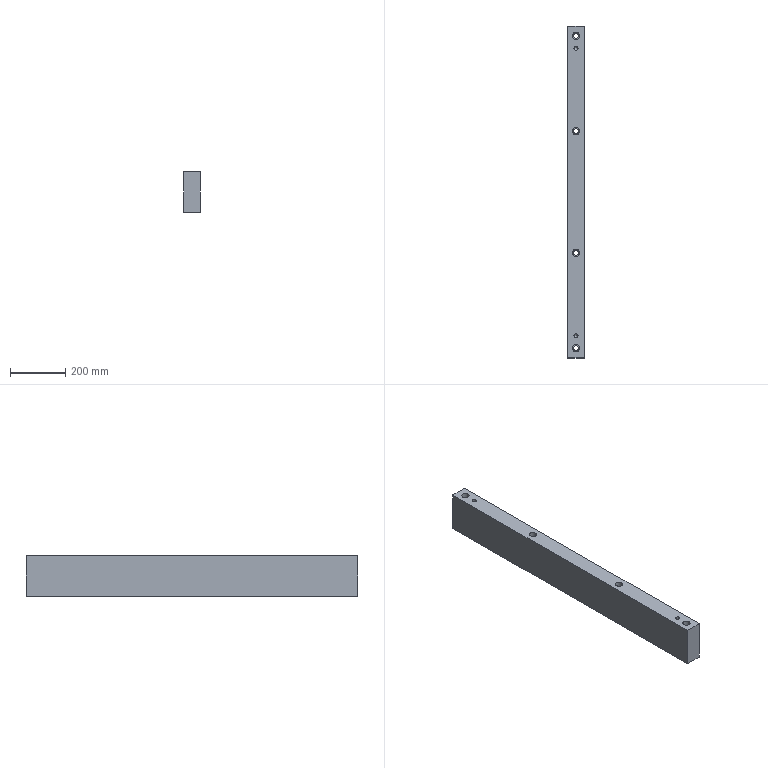Part | STEP file | lll_id1774_x_t | 1 solid | 22 faces | box 60 x 1200 x 147.5 mm | volume 10381772 mm3 | plane 10 | cylinder 10 | cone 2 | commonest cylinder face diameters 18.009 x4 26.008 x4 14.506 x2
STEP:
#1=CARTESIAN_POINT('',(1069.688,-520.,370.));
#2=VERTEX_POINT('',#1);
#3=CARTESIAN_POINT('',(1062.435,-520.,370.));
#4=DIRECTION('',(0.,0.,-1.));
#5=DIRECTION('',(1.,0.,0.));
#6=AXIS2_PLACEMENT_3D('',#3,#4,#5);
#7=CIRCLE('',#6,7.253);
#8=EDGE_CURVE('',#2,#2,#7,.T.);
#9=ORIENTED_EDGE('',*,*,#8,.T.);
#10=EDGE_LOOP('',(#9));
#11=FACE_BOUND('',#10,.T.);
#12=CARTESIAN_POINT('',(1069.688,520.,370.));
#13=VERTEX_POINT('',#12);
#14=CARTESIAN_POINT('',(1062.435,520.,370.));
#15=DIRECTION('',(0.,0.,1.));
#16=DIRECTION('',(1.,0.,0.));
#17=AXIS2_PLACEMENT_3D('',#14,#15,#16);
#18=CIRCLE('',#17,7.253);
#19=EDGE_CURVE('',#13,#13,#18,.T.);
#20=ORIENTED_EDGE('',*,*,#19,.F.);
#21=EDGE_LOOP('',(#20));
#22=FACE_BOUND('',#21,.T.);
#23=CARTESIAN_POINT('',(1075.439,565.,370.));
#24=VERTEX_POINT('',#23);
#25=CARTESIAN_POINT('',(1062.435,565.,370.));
#26=DIRECTION('',(0.,0.,1.));
#27=DIRECTION('',(1.,0.,0.));
#28=AXIS2_PLACEMENT_3D('',#25,#26,#27);
#29=CIRCLE('',#28,13.004);
#30=EDGE_CURVE('',#24,#24,#29,.T.);
#31=ORIENTED_EDGE('',*,*,#30,.F.);
#32=EDGE_LOOP('',(#31));
#33=FACE_BOUND('',#32,.T.);
#34=CARTESIAN_POINT('',(1032.435,600.,370.));
#35=VERTEX_POINT('',#34);
#36=CARTESIAN_POINT('',(1092.435,600.,370.));
#37=VERTEX_POINT('',#36);
#38=CARTESIAN_POINT('',(3278.751,600.,370.));
#39=DIRECTION('',(1.,0.,0.));
#40=VECTOR('',#39,1.);
#41=LINE('',#38,#40);
#42=EDGE_CURVE('',#35,#37,#41,.T.);
#43=ORIENTED_EDGE('',*,*,#42,.F.);
#44=CARTESIAN_POINT('',(1032.435,-600.,370.));
#45=VERTEX_POINT('',#44);
#46=CARTESIAN_POINT('',(1032.435,0.,370.));
#47=DIRECTION('',(0.,1.,0.));
#48=VECTOR('',#47,1.);
#49=LINE('',#46,#48);
#50=EDGE_CURVE('',#45,#35,#49,.T.);
#51=ORIENTED_EDGE('',*,*,#50,.F.);
#52=CARTESIAN_POINT('',(1092.435,-600.,370.));
#53=VERTEX_POINT('',#52);
#54=CARTESIAN_POINT('',(3278.751,-600.,370.));
#55=DIRECTION('',(-1.,0.,0.));
#56=VECTOR('',#55,1.);
#57=LINE('',#54,#56);
#58=EDGE_CURVE('',#53,#45,#57,.T.);
#59=ORIENTED_EDGE('',*,*,#58,.F.);
#60=CARTESIAN_POINT('',(1092.435,1.,370.));
#61=DIRECTION('',(0.,-1.,0.));
#62=VECTOR('',#61,1.);
#63=LINE('',#60,#62);
#64=EDGE_CURVE('',#37,#53,#63,.T.);
#65=ORIENTED_EDGE('',*,*,#64,.F.);
#66=EDGE_LOOP('',(#43,#51,#59,#65));
#67=FACE_BOUND('',#66,.T.);
#68=CARTESIAN_POINT('',(1075.439,-565.,370.));
#69=VERTEX_POINT('',#68);
#70=CARTESIAN_POINT('',(1062.435,-565.,370.));
#71=DIRECTION('',(0.,0.,-1.));
#72=DIRECTION('',(1.,0.,0.));
#73=AXIS2_PLACEMENT_3D('',#70,#71,#72);
#74=CIRCLE('',#73,13.004);
#75=EDGE_CURVE('',#69,#69,#74,.T.);
#76=ORIENTED_EDGE('',*,*,#75,.T.);
#77=EDGE_LOOP('',(#76));
#78=FACE_BOUND('',#77,.T.);
#79=CARTESIAN_POINT('',(1075.439,-220.,370.));
#80=VERTEX_POINT('',#79);
#81=CARTESIAN_POINT('',(1062.435,-220.,370.));
#82=DIRECTION('',(0.,0.,-1.));
#83=DIRECTION('',(1.,0.,0.));
#84=AXIS2_PLACEMENT_3D('',#81,#82,#83);
#85=CIRCLE('',#84,13.004);
#86=EDGE_CURVE('',#80,#80,#85,.T.);
#87=ORIENTED_EDGE('',*,*,#86,.T.);
#88=EDGE_LOOP('',(#87));
#89=FACE_BOUND('',#88,.T.);
#90=CARTESIAN_POINT('',(1075.439,220.,370.));
#91=VERTEX_POINT('',#90);
#92=CARTESIAN_POINT('',(1062.435,220.,370.));
#93=DIRECTION('',(0.,0.,1.));
#94=DIRECTION('',(1.,0.,0.));
#95=AXIS2_PLACEMENT_3D('',#92,#93,#94);
#96=CIRCLE('',#95,13.004);
#97=EDGE_CURVE('',#91,#91,#96,.T.);
#98=ORIENTED_EDGE('',*,*,#97,.F.);
#99=EDGE_LOOP('',(#98));
#100=FACE_BOUND('',#99,.T.);
#101=CARTESIAN_POINT('',(3278.751,1.,370.));
#102=DIRECTION('',(0.,0.,-1.));
#103=DIRECTION('',(-1.,0.,0.));
#104=AXIS2_PLACEMENT_3D('',#101,#102,#103);
#105=PLANE('',#104);
#106=ADVANCED_FACE('',(#11,#22,#33,#67,#78,#89,#100),#105,.F.);
#107=CARTESIAN_POINT('',(1071.44,-220.,222.5));
#108=VERTEX_POINT('',#107);
#109=CARTESIAN_POINT('',(1062.435,-220.,222.5));
#110=DIRECTION('',(0.,0.,1.));
#111=DIRECTION('',(1.,0.,0.));
#112=AXIS2_PLACEMENT_3D('',#109,#110,#111);
#113=CIRCLE('',#112,9.005);
#114=EDGE_CURVE('',#108,#108,#113,.T.);
#115=ORIENTED_EDGE('',*,*,#114,.T.);
#116=EDGE_LOOP('',(#115));
#117=FACE_BOUND('',#116,.T.);
#118=CARTESIAN_POINT('',(1032.435,600.,222.5));
#119=VERTEX_POINT('',#118);
#120=CARTESIAN_POINT('',(1092.435,600.,222.5));
#121=VERTEX_POINT('',#120);
#122=CARTESIAN_POINT('',(-2877.565,600.,222.5));
#123=DIRECTION('',(1.,0.,0.));
#124=VECTOR('',#123,1.);
#125=LINE('',#122,#124);
#126=EDGE_CURVE('',#119,#121,#125,.T.);
#127=ORIENTED_EDGE('',*,*,#126,.T.);
#128=CARTESIAN_POINT('',(1092.435,-600.,222.5));
#129=VERTEX_POINT('',#128);
#130=CARTESIAN_POINT('',(1092.435,600.,222.5));
#131=DIRECTION('',(0.,-1.,0.));
#132=VECTOR('',#131,1.);
#133=LINE('',#130,#132);
#134=EDGE_CURVE('',#121,#129,#133,.T.);
#135=ORIENTED_EDGE('',*,*,#134,.T.);
#136=CARTESIAN_POINT('',(1032.435,-600.,222.5));
#137=VERTEX_POINT('',#136);
#138=CARTESIAN_POINT('',(1092.435,-600.,222.5));
#139=DIRECTION('',(-1.,0.,0.));
#140=VECTOR('',#139,1.);
#141=LINE('',#138,#140);
#142=EDGE_CURVE('',#129,#137,#141,.T.);
#143=ORIENTED_EDGE('',*,*,#142,.T.);
#144=CARTESIAN_POINT('',(1032.435,1.,222.5));
#145=DIRECTION('',(0.,-1.,0.));
#146=VECTOR('',#145,1.);
#147=LINE('',#144,#146);
#148=EDGE_CURVE('',#119,#137,#147,.T.);
#149=ORIENTED_EDGE('',*,*,#148,.F.);
#150=EDGE_LOOP('',(#127,#135,#143,#149));
#151=FACE_BOUND('',#150,.T.);
#152=CARTESIAN_POINT('',(1071.44,-565.,222.5));
#153=VERTEX_POINT('',#152);
#154=CARTESIAN_POINT('',(1062.435,-565.,222.5));
#155=DIRECTION('',(0.,0.,1.));
#156=DIRECTION('',(1.,0.,0.));
#157=AXIS2_PLACEMENT_3D('',#154,#155,#156);
#158=CIRCLE('',#157,9.005);
#159=EDGE_CURVE('',#153,#153,#158,.T.);
#160=ORIENTED_EDGE('',*,*,#159,.T.);
#161=EDGE_LOOP('',(#160));
#162=FACE_BOUND('',#161,.T.);
#163=CARTESIAN_POINT('',(1071.44,220.,222.5));
#164=VERTEX_POINT('',#163);
#165=CARTESIAN_POINT('',(1062.435,220.,222.5));
#166=DIRECTION('',(0.,0.,-1.));
#167=DIRECTION('',(1.,0.,0.));
#168=AXIS2_PLACEMENT_3D('',#165,#166,#167);
#169=CIRCLE('',#168,9.005);
#170=EDGE_CURVE('',#164,#164,#169,.T.);
#171=ORIENTED_EDGE('',*,*,#170,.F.);
#172=EDGE_LOOP('',(#171));
#173=FACE_BOUND('',#172,.T.);
#174=CARTESIAN_POINT('',(1071.44,565.,222.5));
#175=VERTEX_POINT('',#174);
#176=CARTESIAN_POINT('',(1062.435,565.,222.5));
#177=DIRECTION('',(0.,0.,-1.));
#178=DIRECTION('',(1.,0.,0.));
#179=AXIS2_PLACEMENT_3D('',#176,#177,#178);
#180=CIRCLE('',#179,9.005);
#181=EDGE_CURVE('',#175,#175,#180,.T.);
#182=ORIENTED_EDGE('',*,*,#181,.F.);
#183=EDGE_LOOP('',(#182));
#184=FACE_BOUND('',#183,.T.);
#185=CARTESIAN_POINT('',(3278.751,1.,222.5));
#186=DIRECTION('',(0.,0.,-1.));
#187=DIRECTION('',(-1.,0.,0.));
#188=AXIS2_PLACEMENT_3D('',#185,#186,#187);
#189=PLANE('',#188);
#190=ADVANCED_FACE('',(#117,#151,#162,#173,#184),#189,.T.);
#191=ORIENTED_EDGE('',*,*,#134,.F.);
#192=CARTESIAN_POINT('',(1092.435,600.,360.));
#193=DIRECTION('',(0.,0.,-1.));
#194=VECTOR('',#193,1.);
#195=LINE('',#192,#194);
#196=EDGE_CURVE('',#37,#121,#195,.T.);
#197=ORIENTED_EDGE('',*,*,#196,.F.);
#198=ORIENTED_EDGE('',*,*,#64,.T.);
#199=CARTESIAN_POINT('',(1092.435,-600.,360.));
#200=DIRECTION('',(0.,0.,-1.));
#201=VECTOR('',#200,1.);
#202=LINE('',#199,#201);
#203=EDGE_CURVE('',#53,#129,#202,.T.);
#204=ORIENTED_EDGE('',*,*,#203,.T.);
#205=EDGE_LOOP('',(#191,#197,#198,#204));
#206=FACE_OUTER_BOUND('',#205,.T.);
#207=CARTESIAN_POINT('',(1092.435,600.,360.));
#208=DIRECTION('',(1.,0.,0.));
#209=DIRECTION('',(0.,0.,-1.));
#210=AXIS2_PLACEMENT_3D('',#207,#208,#209);
#211=PLANE('',#210);
#212=ADVANCED_FACE('',(#206),#211,.T.);
#213=CARTESIAN_POINT('',(1032.435,-600.,360.));
#214=DIRECTION('',(0.,0.,-1.));
#215=VECTOR('',#214,1.);
#216=LINE('',#213,#215);
#217=EDGE_CURVE('',#45,#137,#216,.T.);
#218=ORIENTED_EDGE('',*,*,#217,.T.);
#219=ORIENTED_EDGE('',*,*,#142,.F.);
#220=ORIENTED_EDGE('',*,*,#203,.F.);
#221=ORIENTED_EDGE('',*,*,#58,.T.);
#222=EDGE_LOOP('',(#218,#219,#220,#221));
#223=FACE_OUTER_BOUND('',#222,.T.);
#224=CARTESIAN_POINT('',(1092.435,-600.,360.));
#225=DIRECTION('',(0.,-1.,0.));
#226=DIRECTION('',(0.,0.,-1.));
#227=AXIS2_PLACEMENT_3D('',#224,#225,#226);
#228=PLANE('',#227);
#229=ADVANCED_FACE('',(#223),#228,.T.);
#230=CARTESIAN_POINT('',(1032.435,600.,360.));
#231=DIRECTION('',(0.,0.,1.));
#232=VECTOR('',#231,1.);
#233=LINE('',#230,#232);
#234=EDGE_CURVE('',#119,#35,#233,.T.);
#235=ORIENTED_EDGE('',*,*,#234,.T.);
#236=ORIENTED_EDGE('',*,*,#42,.T.);
#237=ORIENTED_EDGE('',*,*,#196,.T.);
#238=ORIENTED_EDGE('',*,*,#126,.F.);
#239=EDGE_LOOP('',(#235,#236,#237,#238));
#240=FACE_OUTER_BOUND('',#239,.T.);
#241=CARTESIAN_POINT('',(-2877.565,600.,360.));
#242=DIRECTION('',(0.,1.,0.));
#243=DIRECTION('',(0.,0.,1.));
#244=AXIS2_PLACEMENT_3D('',#241,#242,#243);
#245=PLANE('',#244);
#246=ADVANCED_FACE('',(#240),#245,.T.);
#247=ORIENTED_EDGE('',*,*,#148,.T.);
#248=ORIENTED_EDGE('',*,*,#217,.F.);
#249=ORIENTED_EDGE('',*,*,#50,.T.);
#250=ORIENTED_EDGE('',*,*,#234,.F.);
#251=EDGE_LOOP('',(#247,#248,#249,#250));
#252=FACE_OUTER_BOUND('',#251,.T.);
#253=CARTESIAN_POINT('',(1032.435,0.,291.25));
#254=DIRECTION('',(1.,0.,0.));
#255=DIRECTION('',(0.,0.,-1.));
#256=AXIS2_PLACEMENT_3D('',#253,#254,#255);
#257=PLANE('',#256);
#258=ADVANCED_FACE('',(#252),#257,.F.);
#259=CARTESIAN_POINT('',(1071.44,-565.,302.5));
#260=VERTEX_POINT('',#259);
#261=CARTESIAN_POINT('',(1062.435,-565.,302.5));
#262=DIRECTION('',(0.,0.,-1.));
#263=DIRECTION('',(1.,0.,0.));
#264=AXIS2_PLACEMENT_3D('',#261,#262,#263);
#265=CIRCLE('',#264,9.005);
#266=EDGE_CURVE('',#260,#260,#265,.T.);
#267=ORIENTED_EDGE('',*,*,#266,.F.);
#268=EDGE_LOOP('',(#267));
#269=FACE_BOUND('',#268,.T.);
#270=ORIENTED_EDGE('',*,*,#159,.F.);
#271=EDGE_LOOP('',(#270));
#272=FACE_BOUND('',#271,.T.);
#273=CARTESIAN_POINT('',(1062.435,-565.,420.));
#274=DIRECTION('',(0.,0.,-1.));
#275=DIRECTION('',(1.,0.,0.));
#276=AXIS2_PLACEMENT_3D('',#273,#274,#275);
#277=CYLINDRICAL_SURFACE('',#276,9.005);
#278=ADVANCED_FACE('',(#269,#272),#277,.F.);
#279=ORIENTED_EDGE('',*,*,#266,.T.);
#280=EDGE_LOOP('',(#279));
#281=FACE_BOUND('',#280,.T.);
#282=CARTESIAN_POINT('',(1075.439,-565.,302.5));
#283=VERTEX_POINT('',#282);
#284=CARTESIAN_POINT('',(1062.435,-565.,302.5));
#285=DIRECTION('',(0.,0.,-1.));
#286=DIRECTION('',(1.,0.,0.));
#287=AXIS2_PLACEMENT_3D('',#284,#285,#286);
#288=CIRCLE('',#287,13.004);
#289=EDGE_CURVE('',#283,#283,#288,.T.);
#290=ORIENTED_EDGE('',*,*,#289,.F.);
#291=EDGE_LOOP('',(#290));
#292=FACE_BOUND('',#291,.T.);
#293=CARTESIAN_POINT('',(2132.435,0.,302.5));
#294=DIRECTION('',(0.,0.,1.));
#295=DIRECTION('',(1.,0.,0.));
#296=AXIS2_PLACEMENT_3D('',#293,#294,#295);
#297=PLANE('',#296);
#298=ADVANCED_FACE('',(#281,#292),#297,.T.);
#299=ORIENTED_EDGE('',*,*,#289,.T.);
#300=EDGE_LOOP('',(#299));
#301=FACE_BOUND('',#300,.T.);
#302=ORIENTED_EDGE('',*,*,#75,.F.);
#303=EDGE_LOOP('',(#302));
#304=FACE_BOUND('',#303,.T.);
#305=CARTESIAN_POINT('',(1062.435,-565.,420.));
#306=DIRECTION('',(0.,0.,-1.));
#307=DIRECTION('',(1.,0.,0.));
#308=AXIS2_PLACEMENT_3D('',#305,#306,#307);
#309=CYLINDRICAL_SURFACE('',#308,13.004);
#310=ADVANCED_FACE('',(#301,#304),#309,.F.);
#311=CARTESIAN_POINT('',(1071.44,-220.,302.5));
#312=VERTEX_POINT('',#311);
#313=CARTESIAN_POINT('',(1062.435,-220.,302.5));
#314=DIRECTION('',(0.,0.,-1.));
#315=DIRECTION('',(1.,0.,0.));
#316=AXIS2_PLACEMENT_3D('',#313,#314,#315);
#317=CIRCLE('',#316,9.005);
#318=EDGE_CURVE('',#312,#312,#317,.T.);
#319=ORIENTED_EDGE('',*,*,#318,.F.);
#320=EDGE_LOOP('',(#319));
#321=FACE_BOUND('',#320,.T.);
#322=ORIENTED_EDGE('',*,*,#114,.F.);
#323=EDGE_LOOP('',(#322));
#324=FACE_BOUND('',#323,.T.);
#325=CARTESIAN_POINT('',(1062.435,-220.,420.));
#326=DIRECTION('',(0.,0.,-1.));
#327=DIRECTION('',(1.,0.,0.));
#328=AXIS2_PLACEMENT_3D('',#325,#326,#327);
#329=CYLINDRICAL_SURFACE('',#328,9.005);
#330=ADVANCED_FACE('',(#321,#324),#329,.F.);
#331=ORIENTED_EDGE('',*,*,#318,.T.);
#332=EDGE_LOOP('',(#331));
#333=FACE_BOUND('',#332,.T.);
#334=CARTESIAN_POINT('',(1075.439,-220.,302.5));
#335=VERTEX_POINT('',#334);
#336=CARTESIAN_POINT('',(1062.435,-220.,302.5));
#337=DIRECTION('',(0.,0.,-1.));
#338=DIRECTION('',(1.,0.,0.));
#339=AXIS2_PLACEMENT_3D('',#336,#337,#338);
#340=CIRCLE('',#339,13.004);
#341=EDGE_CURVE('',#335,#335,#340,.T.);
#342=ORIENTED_EDGE('',*,*,#341,.F.);
#343=EDGE_LOOP('',(#342));
#344=FACE_BOUND('',#343,.T.);
#345=CARTESIAN_POINT('',(2132.435,0.,302.5));
#346=DIRECTION('',(0.,0.,1.));
#347=DIRECTION('',(1.,0.,0.));
#348=AXIS2_PLACEMENT_3D('',#345,#346,#347);
#349=PLANE('',#348);
#350=ADVANCED_FACE('',(#333,#344),#349,.T.);
#351=ORIENTED_EDGE('',*,*,#341,.T.);
#352=EDGE_LOOP('',(#351));
#353=FACE_BOUND('',#352,.T.);
#354=ORIENTED_EDGE('',*,*,#86,.F.);
#355=EDGE_LOOP('',(#354));
#356=FACE_BOUND('',#355,.T.);
#357=CARTESIAN_POINT('',(1062.435,-220.,420.));
#358=DIRECTION('',(0.,0.,-1.));
#359=DIRECTION('',(1.,0.,0.));
#360=AXIS2_PLACEMENT_3D('',#357,#358,#359);
#361=CYLINDRICAL_SURFACE('',#360,13.004);
#362=ADVANCED_FACE('',(#353,#356),#361,.F.);
#363=CARTESIAN_POINT('',(1071.44,220.,302.5));
#364=VERTEX_POINT('',#363);
#365=CARTESIAN_POINT('',(1062.435,220.,302.5));
#366=DIRECTION('',(0.,0.,1.));
#367=DIRECTION('',(1.,0.,0.));
#368=AXIS2_PLACEMENT_3D('',#365,#366,#367);
#369=CIRCLE('',#368,9.005);
#370=EDGE_CURVE('',#364,#364,#369,.T.);
#371=ORIENTED_EDGE('',*,*,#370,.T.);
#372=EDGE_LOOP('',(#371));
#373=FACE_BOUND('',#372,.T.);
#374=ORIENTED_EDGE('',*,*,#170,.T.);
#375=EDGE_LOOP('',(#374));
#376=FACE_BOUND('',#375,.T.);
#377=CARTESIAN_POINT('',(1062.435,220.,420.));
#378=DIRECTION('',(0.,0.,-1.));
#379=DIRECTION('',(1.,0.,0.));
#380=AXIS2_PLACEMENT_3D('',#377,#378,#379);
#381=CYLINDRICAL_SURFACE('',#380,9.005);
#382=ADVANCED_FACE('',(#373,#376),#381,.F.);
#383=ORIENTED_EDGE('',*,*,#370,.F.);
#384=EDGE_LOOP('',(#383));
#385=FACE_BOUND('',#384,.T.);
#386=CARTESIAN_POINT('',(1075.439,220.,302.5));
#387=VERTEX_POINT('',#386);
#388=CARTESIAN_POINT('',(1062.435,220.,302.5));
#389=DIRECTION('',(0.,0.,1.));
#390=DIRECTION('',(1.,0.,0.));
#391=AXIS2_PLACEMENT_3D('',#388,#389,#390);
#392=CIRCLE('',#391,13.004);
#393=EDGE_CURVE('',#387,#387,#392,.T.);
#394=ORIENTED_EDGE('',*,*,#393,.T.);
#395=EDGE_LOOP('',(#394));
#396=FACE_BOUND('',#395,.T.);
#397=CARTESIAN_POINT('',(2132.435,0.,302.5));
#398=DIRECTION('',(0.,0.,1.));
#399=DIRECTION('',(1.,0.,0.));
#400=AXIS2_PLACEMENT_3D('',#397,#398,#399);
#401=PLANE('',#400);
#402=ADVANCED_FACE('',(#385,#396),#401,.T.);
#403=ORIENTED_EDGE('',*,*,#393,.F.);
#404=EDGE_LOOP('',(#403));
#405=FACE_BOUND('',#404,.T.);
#406=ORIENTED_EDGE('',*,*,#97,.T.);
#407=EDGE_LOOP('',(#406));
#408=FACE_BOUND('',#407,.T.);
#409=CARTESIAN_POINT('',(1062.435,220.,420.));
#410=DIRECTION('',(0.,0.,-1.));
#411=DIRECTION('',(1.,0.,0.));
#412=AXIS2_PLACEMENT_3D('',#409,#410,#411);
#413=CYLINDRICAL_SURFACE('',#412,13.004);
#414=ADVANCED_FACE('',(#405,#408),#413,.F.);
#415=CARTESIAN_POINT('',(1071.44,565.,302.5));
#416=VERTEX_POINT('',#415);
#417=CARTESIAN_POINT('',(1062.435,565.,302.5));
#418=DIRECTION('',(0.,0.,1.));
#419=DIRECTION('',(1.,0.,0.));
#420=AXIS2_PLACEMENT_3D('',#417,#418,#419);
#421=CIRCLE('',#420,9.005);
#422=EDGE_CURVE('',#416,#416,#421,.T.);
#423=ORIENTED_EDGE('',*,*,#422,.T.);
#424=EDGE_LOOP('',(#423));
#425=FACE_BOUND('',#424,.T.);
#426=ORIENTED_EDGE('',*,*,#181,.T.);
#427=EDGE_LOOP('',(#426));
#428=FACE_BOUND('',#427,.T.);
#429=CARTESIAN_POINT('',(1062.435,565.,420.));
#430=DIRECTION('',(0.,0.,-1.));
#431=DIRECTION('',(1.,0.,0.));
#432=AXIS2_PLACEMENT_3D('',#429,#430,#431);
#433=CYLINDRICAL_SURFACE('',#432,9.005);
#434=ADVANCED_FACE('',(#425,#428),#433,.F.);
#435=ORIENTED_EDGE('',*,*,#422,.F.);
#436=EDGE_LOOP('',(#435));
#437=FACE_BOUND('',#436,.T.);
#438=CARTESIAN_POINT('',(1075.439,565.,302.5));
#439=VERTEX_POINT('',#438);
#440=CARTESIAN_POINT('',(1062.435,565.,302.5));
#441=DIRECTION('',(0.,0.,1.));
#442=DIRECTION('',(1.,0.,0.));
#443=AXIS2_PLACEMENT_3D('',#440,#441,#442);
#444=CIRCLE('',#443,13.004);
#445=EDGE_CURVE('',#439,#439,#444,.T.);
#446=ORIENTED_EDGE('',*,*,#445,.T.);
#447=EDGE_LOOP('',(#446));
#448=FACE_BOUND('',#447,.T.);
#449=CARTESIAN_POINT('',(2132.435,0.,302.5));
#450=DIRECTION('',(0.,0.,1.));
#451=DIRECTION('',(1.,0.,0.));
#452=AXIS2_PLACEMENT_3D('',#449,#450,#451);
#453=PLANE('',#452);
#454=ADVANCED_FACE('',(#437,#448),#453,.T.);
#455=ORIENTED_EDGE('',*,*,#445,.F.);
#456=EDGE_LOOP('',(#455));
#457=FACE_BOUND('',#456,.T.);
#458=ORIENTED_EDGE('',*,*,#30,.T.);
#459=EDGE_LOOP('',(#458));
#460=FACE_BOUND('',#459,.T.);
#461=CARTESIAN_POINT('',(1062.435,565.,420.));
#462=DIRECTION('',(0.,0.,-1.));
#463=DIRECTION('',(1.,0.,0.));
#464=AXIS2_PLACEMENT_3D('',#461,#462,#463);
#465=CYLINDRICAL_SURFACE('',#464,13.004);
#466=ADVANCED_FACE('',(#457,#460),#465,.F.);
#467=CARTESIAN_POINT('',(1055.182,520.,332.247));
#468=VERTEX_POINT('',#467);
#469=CARTESIAN_POINT('',(1062.435,520.,332.247));
#470=DIRECTION('',(0.,0.,1.));
#471=DIRECTION('',(-1.,0.,0.));
#472=AXIS2_PLACEMENT_3D('',#469,#470,#471);
#473=CIRCLE('',#472,7.253);
#474=EDGE_CURVE('',#468,#468,#473,.T.);
#475=ORIENTED_EDGE('',*,*,#474,.F.);
#476=EDGE_LOOP('',(#475));
#477=FACE_BOUND('',#476,.T.);
#478=ORIENTED_EDGE('',*,*,#19,.T.);
#479=EDGE_LOOP('',(#478));
#480=FACE_BOUND('',#479,.T.);
#481=CARTESIAN_POINT('',(1062.435,520.,370.));
#482=DIRECTION('',(0.,0.,-1.));
#483=DIRECTION('',(1.,0.,0.));
#484=AXIS2_PLACEMENT_3D('',#481,#482,#483);
#485=CYLINDRICAL_SURFACE('',#484,7.253);
#486=ADVANCED_FACE('',(#477,#480),#485,.F.);
#487=CARTESIAN_POINT('',(1062.435,520.,324.994));
#488=VERTEX_POINT('',#487);
#489=VERTEX_LOOP('',#488);
#490=FACE_BOUND('',#489,.T.);
#491=ORIENTED_EDGE('',*,*,#474,.T.);
#492=EDGE_LOOP('',(#491));
#493=FACE_BOUND('',#492,.T.);
#494=CARTESIAN_POINT('',(1062.435,520.,332.247));
#495=DIRECTION('',(0.,0.,1.));
#496=DIRECTION('',(1.,0.,0.));
#497=AXIS2_PLACEMENT_3D('',#494,#495,#496);
#498=CONICAL_SURFACE('',#497,7.253,45.);
#499=ADVANCED_FACE('',(#490,#493),#498,.F.);
#500=CARTESIAN_POINT('',(1055.182,-520.,332.247));
#501=VERTEX_POINT('',#500);
#502=CARTESIAN_POINT('',(1062.435,-520.,332.247));
#503=DIRECTION('',(0.,0.,-1.));
#504=DIRECTION('',(-1.,0.,0.));
#505=AXIS2_PLACEMENT_3D('',#502,#503,#504);
#506=CIRCLE('',#505,7.253);
#507=EDGE_CURVE('',#501,#501,#506,.T.);
#508=ORIENTED_EDGE('',*,*,#507,.T.);
#509=EDGE_LOOP('',(#508));
#510=FACE_BOUND('',#509,.T.);
#511=ORIENTED_EDGE('',*,*,#8,.F.);
#512=EDGE_LOOP('',(#511));
#513=FACE_BOUND('',#512,.T.);
#514=CARTESIAN_POINT('',(1062.435,-520.,370.));
#515=DIRECTION('',(0.,0.,-1.));
#516=DIRECTION('',(1.,0.,0.));
#517=AXIS2_PLACEMENT_3D('',#514,#515,#516);
#518=CYLINDRICAL_SURFACE('',#517,7.253);
#519=ADVANCED_FACE('',(#510,#513),#518,.F.);
#520=CARTESIAN_POINT('',(1062.435,-520.,324.994));
#521=VERTEX_POINT('',#520);
#522=VERTEX_LOOP('',#521);
#523=FACE_BOUND('',#522,.T.);
#524=ORIENTED_EDGE('',*,*,#507,.F.);
#525=EDGE_LOOP('',(#524));
#526=FACE_BOUND('',#525,.T.);
#527=CARTESIAN_POINT('',(1062.435,-520.,332.247));
#528=DIRECTION('',(0.,0.,1.));
#529=DIRECTION('',(1.,0.,0.));
#530=AXIS2_PLACEMENT_3D('',#527,#528,#529);
#531=CONICAL_SURFACE('',#530,7.253,45.);
#532=ADVANCED_FACE('',(#523,#526),#531,.F.);
#533=CLOSED_SHELL('',(#106,#190,#212,#229,#246,#258,#278,#298,#310,#330,#350,#362,#382,#402,#414,#434,#454,#466,#486,#499,#519,#532));
#534=MANIFOLD_SOLID_BREP('',#533);
#535=(LENGTH_UNIT()NAMED_UNIT(*)SI_UNIT(.MILLI.,.METRE.));
#536=UNCERTAINTY_MEASURE_WITH_UNIT(LENGTH_MEASURE(0.00002),#535,'','');
#537=(NAMED_UNIT(*)PLANE_ANGLE_UNIT()SI_UNIT($,.RADIAN.));
#538=PLANE_ANGLE_MEASURE_WITH_UNIT(PLANE_ANGLE_MEASURE(0.01745),#537);
#539=DIMENSIONAL_EXPONENTS(0.,0.,0.,0.,0.,0.,0.);
#540=(CONVERSION_BASED_UNIT('DEGREE',#538)NAMED_UNIT(#539)PLANE_ANGLE_UNIT());
#541=(NAMED_UNIT(*)SI_UNIT($,.STERADIAN.)SOLID_ANGLE_UNIT());
#542=(GEOMETRIC_REPRESENTATION_CONTEXT(3)GLOBAL_UNCERTAINTY_ASSIGNED_CONTEXT((#536))GLOBAL_UNIT_ASSIGNED_CONTEXT((#535,#540,#541))REPRESENTATION_CONTEXT('',''));
#543=ADVANCED_BREP_SHAPE_REPRESENTATION('',(#534),#542);